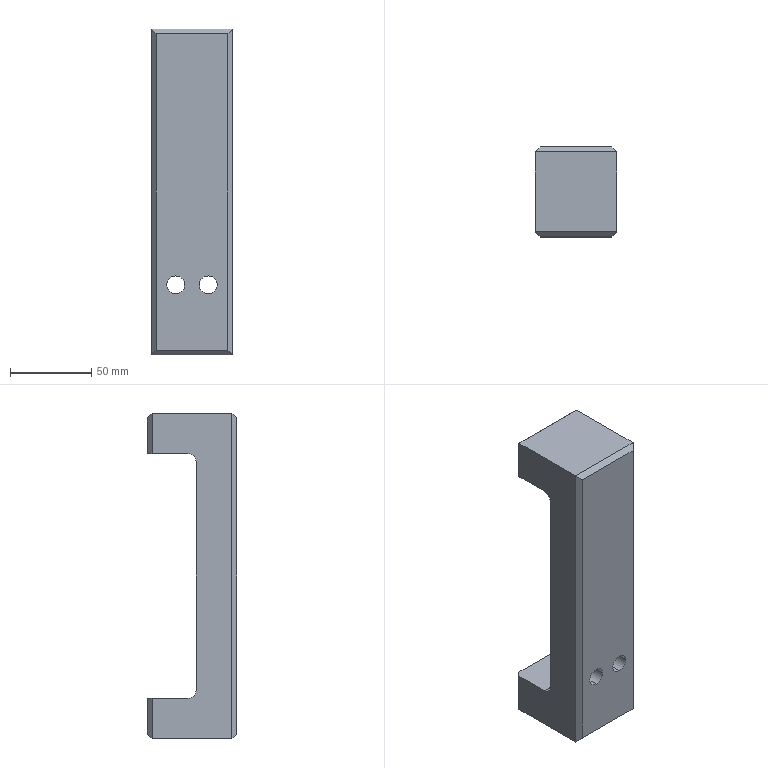Part | CATIA | 1 solid | 26 faces | box 50 x 55 x 200 mm | volume 317707 mm3 | plane 20 | cylinder 6 | commonest cylinder face diameters 11 x4 10 x2
STEP:
#1=CARTESIAN_POINT('',(-22.,-25.,172.));
#2=VERTEX_POINT('',#1);
#3=CARTESIAN_POINT('',(-25.,-22.,175.));
#4=VERTEX_POINT('',#3);
#5=CARTESIAN_POINT('',(-25.,-22.,175.));
#6=CARTESIAN_POINT('',(-22.,-25.,172.));
#7=B_SPLINE_CURVE_WITH_KNOTS('',1,(#5,#6),.UNSPECIFIED.,.F.,.U.,(2,2),(-2.598,2.598),.UNSPECIFIED.);
#8=EDGE_CURVE('',#2,#4,#7,.F.);
#9=ORIENTED_EDGE('',*,*,#8,.T.);
#10=CARTESIAN_POINT('',(-25.,-22.,-25.));
#11=VERTEX_POINT('',#10);
#12=CARTESIAN_POINT('',(-25.,-22.,75.));
#13=DIRECTION('',(0.,0.,1.));
#14=VECTOR('',#13,1.);
#15=LINE('',#12,#14);
#16=EDGE_CURVE('',#11,#4,#15,.T.);
#17=ORIENTED_EDGE('',*,*,#16,.F.);
#18=CARTESIAN_POINT('',(-22.,-25.,-22.));
#19=VERTEX_POINT('',#18);
#20=CARTESIAN_POINT('',(-25.,-22.,-25.));
#21=CARTESIAN_POINT('',(-22.,-25.,-22.));
#22=B_SPLINE_CURVE_WITH_KNOTS('',1,(#20,#21),.UNSPECIFIED.,.F.,.U.,(2,2),(-2.598,2.598),.UNSPECIFIED.);
#23=EDGE_CURVE('',#11,#19,#22,.T.);
#24=ORIENTED_EDGE('',*,*,#23,.T.);
#25=CARTESIAN_POINT('',(-22.,-25.,75.));
#26=DIRECTION('',(0.,0.,1.));
#27=VECTOR('',#26,1.);
#28=LINE('',#25,#27);
#29=EDGE_CURVE('',#19,#2,#28,.T.);
#30=ORIENTED_EDGE('',*,*,#29,.T.);
#31=EDGE_LOOP('',(#9,#17,#24,#30));
#32=FACE_OUTER_BOUND('',#31,.T.);
#33=CARTESIAN_POINT('',(-22.,-25.,-65.));
#34=DIRECTION('',(-0.7071,-0.7071,0.));
#35=DIRECTION('',(0.,0.,1.));
#36=AXIS2_PLACEMENT_3D('',#33,#34,#35);
#37=PLANE('',#36);
#38=ADVANCED_FACE('',(#32),#37,.T.);
#39=CARTESIAN_POINT('',(22.,-25.,172.));
#40=VERTEX_POINT('',#39);
#41=CARTESIAN_POINT('',(25.,-22.,175.));
#42=VERTEX_POINT('',#41);
#43=CARTESIAN_POINT('',(25.,-22.,175.));
#44=CARTESIAN_POINT('',(22.,-25.,172.));
#45=B_SPLINE_CURVE_WITH_KNOTS('',1,(#43,#44),.UNSPECIFIED.,.F.,.U.,(2,2),(-2.598,2.598),.UNSPECIFIED.);
#46=EDGE_CURVE('',#40,#42,#45,.F.);
#47=ORIENTED_EDGE('',*,*,#46,.T.);
#48=CARTESIAN_POINT('',(0.,-22.,175.));
#49=DIRECTION('',(1.,0.,0.));
#50=VECTOR('',#49,1.);
#51=LINE('',#48,#50);
#52=EDGE_CURVE('',#4,#42,#51,.T.);
#53=ORIENTED_EDGE('',*,*,#52,.F.);
#54=ORIENTED_EDGE('',*,*,#8,.F.);
#55=CARTESIAN_POINT('',(0.,-25.,172.));
#56=DIRECTION('',(1.,0.,0.));
#57=VECTOR('',#56,1.);
#58=LINE('',#55,#57);
#59=EDGE_CURVE('',#2,#40,#58,.T.);
#60=ORIENTED_EDGE('',*,*,#59,.T.);
#61=EDGE_LOOP('',(#47,#53,#54,#60));
#62=FACE_OUTER_BOUND('',#61,.T.);
#63=CARTESIAN_POINT('',(-35.,-25.,172.));
#64=DIRECTION('',(0.,-0.7071,0.7071));
#65=DIRECTION('',(1.,0.,0.));
#66=AXIS2_PLACEMENT_3D('',#63,#64,#65);
#67=PLANE('',#66);
#68=ADVANCED_FACE('',(#62),#67,.T.);
#69=CARTESIAN_POINT('',(25.,-22.,-25.));
#70=VERTEX_POINT('',#69);
#71=CARTESIAN_POINT('',(25.,-22.,75.));
#72=DIRECTION('',(0.,0.,1.));
#73=VECTOR('',#72,1.);
#74=LINE('',#71,#73);
#75=EDGE_CURVE('',#42,#70,#74,.F.);
#76=ORIENTED_EDGE('',*,*,#75,.F.);
#77=ORIENTED_EDGE('',*,*,#46,.F.);
#78=CARTESIAN_POINT('',(22.,-25.,-22.));
#79=VERTEX_POINT('',#78);
#80=CARTESIAN_POINT('',(22.,-25.,75.));
#81=DIRECTION('',(0.,0.,1.));
#82=VECTOR('',#81,1.);
#83=LINE('',#80,#82);
#84=EDGE_CURVE('',#40,#79,#83,.F.);
#85=ORIENTED_EDGE('',*,*,#84,.T.);
#86=CARTESIAN_POINT('',(25.,-22.,-25.));
#87=CARTESIAN_POINT('',(22.,-25.,-22.));
#88=B_SPLINE_CURVE_WITH_KNOTS('',1,(#86,#87),.UNSPECIFIED.,.F.,.U.,(2,2),(-2.598,2.598),.UNSPECIFIED.);
#89=EDGE_CURVE('',#79,#70,#88,.F.);
#90=ORIENTED_EDGE('',*,*,#89,.T.);
#91=EDGE_LOOP('',(#76,#77,#85,#90));
#92=FACE_OUTER_BOUND('',#91,.T.);
#93=CARTESIAN_POINT('',(22.,-25.,-65.));
#94=DIRECTION('',(-0.7071,0.7071,0.));
#95=DIRECTION('',(0.,0.,1.));
#96=AXIS2_PLACEMENT_3D('',#93,#94,#95);
#97=PLANE('',#96);
#98=ADVANCED_FACE('',(#92),#97,.F.);
#99=ORIENTED_EDGE('',*,*,#23,.F.);
#100=CARTESIAN_POINT('',(0.,-22.,-25.));
#101=DIRECTION('',(-1.,0.,0.));
#102=VECTOR('',#101,1.);
#103=LINE('',#100,#102);
#104=EDGE_CURVE('',#70,#11,#103,.T.);
#105=ORIENTED_EDGE('',*,*,#104,.F.);
#106=ORIENTED_EDGE('',*,*,#89,.F.);
#107=CARTESIAN_POINT('',(0.,-25.,-22.));
#108=DIRECTION('',(-1.,0.,0.));
#109=VECTOR('',#108,1.);
#110=LINE('',#107,#109);
#111=EDGE_CURVE('',#79,#19,#110,.T.);
#112=ORIENTED_EDGE('',*,*,#111,.T.);
#113=EDGE_LOOP('',(#99,#105,#106,#112));
#114=FACE_OUTER_BOUND('',#113,.T.);
#115=CARTESIAN_POINT('',(35.,-25.,-22.));
#116=DIRECTION('',(0.,-0.7071,-0.7071));
#117=DIRECTION('',(-1.,0.,0.));
#118=AXIS2_PLACEMENT_3D('',#115,#116,#117);
#119=PLANE('',#118);
#120=ADVANCED_FACE('',(#114),#119,.T.);
#121=CARTESIAN_POINT('',(-22.,30.,150.));
#122=VERTEX_POINT('',#121);
#123=CARTESIAN_POINT('',(22.,30.,150.));
#124=VERTEX_POINT('',#123);
#125=CARTESIAN_POINT('',(0.,30.,150.));
#126=DIRECTION('',(1.,0.,0.));
#127=VECTOR('',#126,1.);
#128=LINE('',#125,#127);
#129=EDGE_CURVE('',#122,#124,#128,.T.);
#130=ORIENTED_EDGE('',*,*,#129,.F.);
#131=CARTESIAN_POINT('',(-22.,30.,172.));
#132=VERTEX_POINT('',#131);
#133=CARTESIAN_POINT('',(-22.,30.,161.));
#134=DIRECTION('',(0.,0.,-1.));
#135=VECTOR('',#134,1.);
#136=LINE('',#133,#135);
#137=EDGE_CURVE('',#132,#122,#136,.T.);
#138=ORIENTED_EDGE('',*,*,#137,.F.);
#139=CARTESIAN_POINT('',(22.,30.,172.));
#140=VERTEX_POINT('',#139);
#141=CARTESIAN_POINT('',(0.,30.,172.));
#142=DIRECTION('',(-1.,0.,0.));
#143=VECTOR('',#142,1.);
#144=LINE('',#141,#143);
#145=EDGE_CURVE('',#140,#132,#144,.T.);
#146=ORIENTED_EDGE('',*,*,#145,.F.);
#147=CARTESIAN_POINT('',(22.,30.,161.));
#148=DIRECTION('',(0.,0.,-1.));
#149=VECTOR('',#148,1.);
#150=LINE('',#147,#149);
#151=EDGE_CURVE('',#124,#140,#150,.F.);
#152=ORIENTED_EDGE('',*,*,#151,.F.);
#153=EDGE_LOOP('',(#130,#138,#146,#152));
#154=FACE_OUTER_BOUND('',#153,.T.);
#155=CARTESIAN_POINT('',(0.,30.,-25.));
#156=DIRECTION('',(0.,1.,0.));
#157=DIRECTION('',(0.,0.,1.));
#158=AXIS2_PLACEMENT_3D('',#155,#156,#157);
#159=PLANE('',#158);
#160=ADVANCED_FACE('',(#154),#159,.T.);
#161=CARTESIAN_POINT('',(25.,27.,175.));
#162=VERTEX_POINT('',#161);
#163=CARTESIAN_POINT('',(-25.,27.,175.));
#164=VERTEX_POINT('',#163);
#165=CARTESIAN_POINT('',(0.,27.,175.));
#166=DIRECTION('',(-1.,0.,0.));
#167=VECTOR('',#166,1.);
#168=LINE('',#165,#167);
#169=EDGE_CURVE('',#162,#164,#168,.T.);
#170=ORIENTED_EDGE('',*,*,#169,.T.);
#171=CARTESIAN_POINT('',(-25.,2.5,175.));
#172=DIRECTION('',(0.,1.,0.));
#173=VECTOR('',#172,1.);
#174=LINE('',#171,#173);
#175=EDGE_CURVE('',#164,#4,#174,.F.);
#176=ORIENTED_EDGE('',*,*,#175,.T.);
#177=ORIENTED_EDGE('',*,*,#52,.T.);
#178=CARTESIAN_POINT('',(25.,2.5,175.));
#179=DIRECTION('',(0.,1.,0.));
#180=VECTOR('',#179,1.);
#181=LINE('',#178,#180);
#182=EDGE_CURVE('',#162,#42,#181,.F.);
#183=ORIENTED_EDGE('',*,*,#182,.F.);
#184=EDGE_LOOP('',(#170,#176,#177,#183));
#185=FACE_OUTER_BOUND('',#184,.T.);
#186=CARTESIAN_POINT('',(0.,-25.,175.));
#187=DIRECTION('',(0.,0.,-1.));
#188=DIRECTION('',(0.,1.,0.));
#189=AXIS2_PLACEMENT_3D('',#186,#187,#188);
#190=PLANE('',#189);
#191=ADVANCED_FACE('',(#185),#190,.F.);
#192=CARTESIAN_POINT('',(25.,27.,150.));
#193=VERTEX_POINT('',#192);
#194=CARTESIAN_POINT('',(25.,27.,75.));
#195=DIRECTION('',(0.,0.,-1.));
#196=VECTOR('',#195,1.);
#197=LINE('',#194,#196);
#198=EDGE_CURVE('',#193,#162,#197,.F.);
#199=ORIENTED_EDGE('',*,*,#198,.F.);
#200=CARTESIAN_POINT('',(23.5,28.5,150.));
#201=DIRECTION('',(0.7071,-0.7071,0.));
#202=VECTOR('',#201,1.);
#203=LINE('',#200,#202);
#204=EDGE_CURVE('',#193,#124,#203,.F.);
#205=ORIENTED_EDGE('',*,*,#204,.T.);
#206=ORIENTED_EDGE('',*,*,#151,.T.);
#207=CARTESIAN_POINT('',(25.,27.,175.));
#208=CARTESIAN_POINT('',(22.,30.,172.));
#209=B_SPLINE_CURVE_WITH_KNOTS('',1,(#207,#208),.UNSPECIFIED.,.F.,.U.,(2,2),(-2.598,2.598),.UNSPECIFIED.);
#210=EDGE_CURVE('',#140,#162,#209,.F.);
#211=ORIENTED_EDGE('',*,*,#210,.T.);
#212=EDGE_LOOP('',(#199,#205,#206,#211));
#213=FACE_OUTER_BOUND('',#212,.T.);
#214=CARTESIAN_POINT('',(22.,30.,215.));
#215=DIRECTION('',(-0.7071,-0.7071,0.));
#216=DIRECTION('',(0.,0.,-1.));
#217=AXIS2_PLACEMENT_3D('',#214,#215,#216);
#218=PLANE('',#217);
#219=ADVANCED_FACE('',(#213),#218,.F.);
#220=CARTESIAN_POINT('',(-25.,27.,175.));
#221=CARTESIAN_POINT('',(-22.,30.,172.));
#222=B_SPLINE_CURVE_WITH_KNOTS('',1,(#220,#221),.UNSPECIFIED.,.F.,.U.,(2,2),(-2.598,2.598),.UNSPECIFIED.);
#223=EDGE_CURVE('',#132,#164,#222,.F.);
#224=ORIENTED_EDGE('',*,*,#223,.T.);
#225=ORIENTED_EDGE('',*,*,#169,.F.);
#226=ORIENTED_EDGE('',*,*,#210,.F.);
#227=ORIENTED_EDGE('',*,*,#145,.T.);
#228=EDGE_LOOP('',(#224,#225,#226,#227));
#229=FACE_OUTER_BOUND('',#228,.T.);
#230=CARTESIAN_POINT('',(35.,30.,172.));
#231=DIRECTION('',(0.,0.7071,0.7071));
#232=DIRECTION('',(-1.,0.,0.));
#233=AXIS2_PLACEMENT_3D('',#230,#231,#232);
#234=PLANE('',#233);
#235=ADVANCED_FACE('',(#229),#234,.T.);
#236=CARTESIAN_POINT('',(-25.,27.,150.));
#237=VERTEX_POINT('',#236);
#238=CARTESIAN_POINT('',(-23.5,28.5,150.));
#239=DIRECTION('',(-0.7071,-0.7071,0.));
#240=VECTOR('',#239,1.);
#241=LINE('',#238,#240);
#242=EDGE_CURVE('',#122,#237,#241,.T.);
#243=ORIENTED_EDGE('',*,*,#242,.T.);
#244=CARTESIAN_POINT('',(-25.,27.,75.));
#245=DIRECTION('',(0.,0.,-1.));
#246=VECTOR('',#245,1.);
#247=LINE('',#244,#246);
#248=EDGE_CURVE('',#164,#237,#247,.T.);
#249=ORIENTED_EDGE('',*,*,#248,.F.);
#250=ORIENTED_EDGE('',*,*,#223,.F.);
#251=ORIENTED_EDGE('',*,*,#137,.T.);
#252=EDGE_LOOP('',(#243,#249,#250,#251));
#253=FACE_OUTER_BOUND('',#252,.T.);
#254=CARTESIAN_POINT('',(-22.,30.,215.));
#255=DIRECTION('',(-0.7071,0.7071,0.));
#256=DIRECTION('',(0.,0.,-1.));
#257=AXIS2_PLACEMENT_3D('',#254,#255,#256);
#258=PLANE('',#257);
#259=ADVANCED_FACE('',(#253),#258,.T.);
#260=CARTESIAN_POINT('',(-22.,30.,0.));
#261=VERTEX_POINT('',#260);
#262=CARTESIAN_POINT('',(22.,30.,0.));
#263=VERTEX_POINT('',#262);
#264=CARTESIAN_POINT('',(0.,30.,0.));
#265=DIRECTION('',(1.,0.,0.));
#266=VECTOR('',#265,1.);
#267=LINE('',#264,#266);
#268=EDGE_CURVE('',#261,#263,#267,.T.);
#269=ORIENTED_EDGE('',*,*,#268,.T.);
#270=CARTESIAN_POINT('',(22.,30.,-22.));
#271=VERTEX_POINT('',#270);
#272=CARTESIAN_POINT('',(22.,30.,-11.));
#273=DIRECTION('',(0.,0.,-1.));
#274=VECTOR('',#273,1.);
#275=LINE('',#272,#274);
#276=EDGE_CURVE('',#263,#271,#275,.T.);
#277=ORIENTED_EDGE('',*,*,#276,.T.);
#278=CARTESIAN_POINT('',(-22.,30.,-22.));
#279=VERTEX_POINT('',#278);
#280=CARTESIAN_POINT('',(0.,30.,-22.));
#281=DIRECTION('',(1.,0.,0.));
#282=VECTOR('',#281,1.);
#283=LINE('',#280,#282);
#284=EDGE_CURVE('',#271,#279,#283,.F.);
#285=ORIENTED_EDGE('',*,*,#284,.T.);
#286=CARTESIAN_POINT('',(-22.,30.,-11.));
#287=DIRECTION('',(0.,0.,-1.));
#288=VECTOR('',#287,1.);
#289=LINE('',#286,#288);
#290=EDGE_CURVE('',#279,#261,#289,.F.);
#291=ORIENTED_EDGE('',*,*,#290,.T.);
#292=EDGE_LOOP('',(#269,#277,#285,#291));
#293=FACE_OUTER_BOUND('',#292,.T.);
#294=ADVANCED_FACE('',(#293),#159,.T.);
#295=CARTESIAN_POINT('',(25.,27.,-25.));
#296=VERTEX_POINT('',#295);
#297=CARTESIAN_POINT('',(-25.,27.,-25.));
#298=VERTEX_POINT('',#297);
#299=CARTESIAN_POINT('',(0.,27.,-25.));
#300=DIRECTION('',(1.,0.,0.));
#301=VECTOR('',#300,1.);
#302=LINE('',#299,#301);
#303=EDGE_CURVE('',#296,#298,#302,.F.);
#304=ORIENTED_EDGE('',*,*,#303,.F.);
#305=CARTESIAN_POINT('',(25.,2.5,-25.));
#306=DIRECTION('',(0.,-1.,0.));
#307=VECTOR('',#306,1.);
#308=LINE('',#305,#307);
#309=EDGE_CURVE('',#70,#296,#308,.F.);
#310=ORIENTED_EDGE('',*,*,#309,.F.);
#311=ORIENTED_EDGE('',*,*,#104,.T.);
#312=CARTESIAN_POINT('',(-25.,2.5,-25.));
#313=DIRECTION('',(0.,-1.,0.));
#314=VECTOR('',#313,1.);
#315=LINE('',#312,#314);
#316=EDGE_CURVE('',#11,#298,#315,.F.);
#317=ORIENTED_EDGE('',*,*,#316,.T.);
#318=EDGE_LOOP('',(#304,#310,#311,#317));
#319=FACE_OUTER_BOUND('',#318,.T.);
#320=CARTESIAN_POINT('',(0.,30.,-25.));
#321=DIRECTION('',(0.,0.,1.));
#322=DIRECTION('',(0.,-1.,0.));
#323=AXIS2_PLACEMENT_3D('',#320,#321,#322);
#324=PLANE('',#323);
#325=ADVANCED_FACE('',(#319),#324,.F.);
#326=ORIENTED_EDGE('',*,*,#276,.F.);
#327=CARTESIAN_POINT('',(25.,27.,0.));
#328=VERTEX_POINT('',#327);
#329=CARTESIAN_POINT('',(23.5,28.5,0.));
#330=DIRECTION('',(0.7071,-0.7071,0.));
#331=VECTOR('',#330,1.);
#332=LINE('',#329,#331);
#333=EDGE_CURVE('',#263,#328,#332,.T.);
#334=ORIENTED_EDGE('',*,*,#333,.T.);
#335=CARTESIAN_POINT('',(25.,27.,75.));
#336=DIRECTION('',(0.,0.,-1.));
#337=VECTOR('',#336,1.);
#338=LINE('',#335,#337);
#339=EDGE_CURVE('',#328,#296,#338,.T.);
#340=ORIENTED_EDGE('',*,*,#339,.T.);
#341=CARTESIAN_POINT('',(25.,27.,-25.));
#342=CARTESIAN_POINT('',(22.,30.,-22.));
#343=B_SPLINE_CURVE_WITH_KNOTS('',1,(#341,#342),.UNSPECIFIED.,.F.,.U.,(2,2),(-2.598,2.598),.UNSPECIFIED.);
#344=EDGE_CURVE('',#296,#271,#343,.T.);
#345=ORIENTED_EDGE('',*,*,#344,.T.);
#346=EDGE_LOOP('',(#326,#334,#340,#345));
#347=FACE_OUTER_BOUND('',#346,.T.);
#348=CARTESIAN_POINT('',(22.,30.,215.));
#349=DIRECTION('',(-0.7071,-0.7071,0.));
#350=DIRECTION('',(0.,0.,-1.));
#351=AXIS2_PLACEMENT_3D('',#348,#349,#350);
#352=PLANE('',#351);
#353=ADVANCED_FACE('',(#347),#352,.F.);
#354=CARTESIAN_POINT('',(-25.,27.,-25.));
#355=CARTESIAN_POINT('',(-22.,30.,-22.));
#356=B_SPLINE_CURVE_WITH_KNOTS('',1,(#354,#355),.UNSPECIFIED.,.F.,.U.,(2,2),(-2.598,2.598),.UNSPECIFIED.);
#357=EDGE_CURVE('',#298,#279,#356,.T.);
#358=ORIENTED_EDGE('',*,*,#357,.T.);
#359=ORIENTED_EDGE('',*,*,#284,.F.);
#360=ORIENTED_EDGE('',*,*,#344,.F.);
#361=ORIENTED_EDGE('',*,*,#303,.T.);
#362=EDGE_LOOP('',(#358,#359,#360,#361));
#363=FACE_OUTER_BOUND('',#362,.T.);
#364=CARTESIAN_POINT('',(-35.,30.,-22.));
#365=DIRECTION('',(0.,0.7071,-0.7071));
#366=DIRECTION('',(1.,0.,0.));
#367=AXIS2_PLACEMENT_3D('',#364,#365,#366);
#368=PLANE('',#367);
#369=ADVANCED_FACE('',(#363),#368,.T.);
#370=CARTESIAN_POINT('',(-25.,27.,0.));
#371=VERTEX_POINT('',#370);
#372=CARTESIAN_POINT('',(-23.5,28.5,0.));
#373=DIRECTION('',(-0.7071,-0.7071,0.));
#374=VECTOR('',#373,1.);
#375=LINE('',#372,#374);
#376=EDGE_CURVE('',#371,#261,#375,.F.);
#377=ORIENTED_EDGE('',*,*,#376,.T.);
#378=ORIENTED_EDGE('',*,*,#290,.F.);
#379=ORIENTED_EDGE('',*,*,#357,.F.);
#380=CARTESIAN_POINT('',(-25.,27.,75.));
#381=DIRECTION('',(0.,0.,-1.));
#382=VECTOR('',#381,1.);
#383=LINE('',#380,#382);
#384=EDGE_CURVE('',#298,#371,#383,.F.);
#385=ORIENTED_EDGE('',*,*,#384,.T.);
#386=EDGE_LOOP('',(#377,#378,#379,#385));
#387=FACE_OUTER_BOUND('',#386,.T.);
#388=CARTESIAN_POINT('',(-22.,30.,215.));
#389=DIRECTION('',(-0.7071,0.7071,0.));
#390=DIRECTION('',(0.,0.,-1.));
#391=AXIS2_PLACEMENT_3D('',#388,#389,#390);
#392=PLANE('',#391);
#393=ADVANCED_FACE('',(#387),#392,.T.);
#394=CARTESIAN_POINT('',(25.,5.,0.));
#395=VERTEX_POINT('',#394);
#396=CARTESIAN_POINT('',(25.,16.,0.));
#397=DIRECTION('',(0.,-1.,0.));
#398=VECTOR('',#397,1.);
#399=LINE('',#396,#398);
#400=EDGE_CURVE('',#328,#395,#399,.T.);
#401=ORIENTED_EDGE('',*,*,#400,.F.);
#402=ORIENTED_EDGE('',*,*,#333,.F.);
#403=ORIENTED_EDGE('',*,*,#268,.F.);
#404=ORIENTED_EDGE('',*,*,#376,.F.);
#405=CARTESIAN_POINT('',(-25.,5.,0.));
#406=VERTEX_POINT('',#405);
#407=CARTESIAN_POINT('',(-25.,16.,0.));
#408=DIRECTION('',(0.,-1.,0.));
#409=VECTOR('',#408,1.);
#410=LINE('',#407,#409);
#411=EDGE_CURVE('',#371,#406,#410,.T.);
#412=ORIENTED_EDGE('',*,*,#411,.T.);
#413=CARTESIAN_POINT('',(0.,5.,0.));
#414=DIRECTION('',(1.,0.,0.));
#415=VECTOR('',#414,1.);
#416=LINE('',#413,#415);
#417=EDGE_CURVE('',#395,#406,#416,.F.);
#418=ORIENTED_EDGE('',*,*,#417,.F.);
#419=EDGE_LOOP('',(#401,#402,#403,#404,#412,#418));
#420=FACE_OUTER_BOUND('',#419,.T.);
#421=CARTESIAN_POINT('',(0.,30.,0.));
#422=DIRECTION('',(0.,0.,1.));
#423=DIRECTION('',(0.,-1.,0.));
#424=AXIS2_PLACEMENT_3D('',#421,#422,#423);
#425=PLANE('',#424);
#426=ADVANCED_FACE('',(#420),#425,.T.);
#427=CARTESIAN_POINT('',(25.,0.,5.));
#428=VERTEX_POINT('',#427);
#429=CARTESIAN_POINT('',(-25.,0.,5.));
#430=VERTEX_POINT('',#429);
#431=CARTESIAN_POINT('',(0.,0.,5.));
#432=DIRECTION('',(1.,0.,0.));
#433=VECTOR('',#432,1.);
#434=LINE('',#431,#433);
#435=EDGE_CURVE('',#428,#430,#434,.F.);
#436=ORIENTED_EDGE('',*,*,#435,.F.);
#437=CARTESIAN_POINT('',(25.,5.,5.));
#438=DIRECTION('',(1.,0.,0.));
#439=AXIS2_PLACEMENT_3D('',#437,#438,$);
#440=CIRCLE('',#439,5.);
#441=EDGE_CURVE('',#395,#428,#440,.F.);
#442=ORIENTED_EDGE('',*,*,#441,.F.);
#443=ORIENTED_EDGE('',*,*,#417,.T.);
#444=CARTESIAN_POINT('',(-25.,5.,5.));
#445=DIRECTION('',(1.,0.,0.));
#446=AXIS2_PLACEMENT_3D('',#444,#445,$);
#447=CIRCLE('',#446,5.);
#448=EDGE_CURVE('',#430,#406,#447,.T.);
#449=ORIENTED_EDGE('',*,*,#448,.F.);
#450=EDGE_LOOP('',(#436,#442,#443,#449));
#451=FACE_OUTER_BOUND('',#450,.T.);
#452=CARTESIAN_POINT('',(0.,5.,5.));
#453=DIRECTION('',(1.,0.,0.));
#454=DIRECTION('',(0.,-1.,0.));
#455=AXIS2_PLACEMENT_3D('',#452,#453,#454);
#456=CYLINDRICAL_SURFACE('',#455,5.);
#457=ADVANCED_FACE('',(#451),#456,.F.);
#458=CARTESIAN_POINT('',(25.,0.,145.));
#459=VERTEX_POINT('',#458);
#460=CARTESIAN_POINT('',(25.,5.,150.));
#461=VERTEX_POINT('',#460);
#462=CARTESIAN_POINT('',(25.,5.,145.));
#463=DIRECTION('',(1.,0.,0.));
#464=AXIS2_PLACEMENT_3D('',#462,#463,$);
#465=CIRCLE('',#464,5.);
#466=EDGE_CURVE('',#459,#461,#465,.F.);
#467=ORIENTED_EDGE('',*,*,#466,.T.);
#468=CARTESIAN_POINT('',(25.,16.,150.));
#469=DIRECTION('',(0.,1.,0.));
#470=VECTOR('',#469,1.);
#471=LINE('',#468,#470);
#472=EDGE_CURVE('',#461,#193,#471,.T.);
#473=ORIENTED_EDGE('',*,*,#472,.T.);
#474=ORIENTED_EDGE('',*,*,#198,.T.);
#475=ORIENTED_EDGE('',*,*,#182,.T.);
#476=ORIENTED_EDGE('',*,*,#75,.T.);
#477=ORIENTED_EDGE('',*,*,#309,.T.);
#478=ORIENTED_EDGE('',*,*,#339,.F.);
#479=ORIENTED_EDGE('',*,*,#400,.T.);
#480=ORIENTED_EDGE('',*,*,#441,.T.);
#481=CARTESIAN_POINT('',(25.,0.,75.));
#482=DIRECTION('',(0.,0.,-1.));
#483=VECTOR('',#482,1.);
#484=LINE('',#481,#483);
#485=EDGE_CURVE('',#428,#459,#484,.F.);
#486=ORIENTED_EDGE('',*,*,#485,.T.);
#487=EDGE_LOOP('',(#467,#473,#474,#475,#476,#477,#478,#479,#480,#486));
#488=FACE_OUTER_BOUND('',#487,.T.);
#489=CARTESIAN_POINT('',(25.,0.,0.));
#490=DIRECTION('',(1.,0.,0.));
#491=DIRECTION('',(0.,1.,0.));
#492=AXIS2_PLACEMENT_3D('',#489,#490,#491);
#493=PLANE('',#492);
#494=ADVANCED_FACE('',(#488),#493,.T.);
#495=CARTESIAN_POINT('',(-25.,0.,145.));
#496=VERTEX_POINT('',#495);
#497=CARTESIAN_POINT('',(-25.,0.,75.));
#498=DIRECTION('',(0.,0.,-1.));
#499=VECTOR('',#498,1.);
#500=LINE('',#497,#499);
#501=EDGE_CURVE('',#430,#496,#500,.F.);
#502=ORIENTED_EDGE('',*,*,#501,.F.);
#503=ORIENTED_EDGE('',*,*,#448,.T.);
#504=ORIENTED_EDGE('',*,*,#411,.F.);
#505=ORIENTED_EDGE('',*,*,#384,.F.);
#506=ORIENTED_EDGE('',*,*,#316,.F.);
#507=ORIENTED_EDGE('',*,*,#16,.T.);
#508=ORIENTED_EDGE('',*,*,#175,.F.);
#509=ORIENTED_EDGE('',*,*,#248,.T.);
#510=CARTESIAN_POINT('',(-25.,5.,150.));
#511=VERTEX_POINT('',#510);
#512=CARTESIAN_POINT('',(-25.,16.,150.));
#513=DIRECTION('',(0.,1.,0.));
#514=VECTOR('',#513,1.);
#515=LINE('',#512,#514);
#516=EDGE_CURVE('',#511,#237,#515,.T.);
#517=ORIENTED_EDGE('',*,*,#516,.F.);
#518=CARTESIAN_POINT('',(-25.,5.,145.));
#519=DIRECTION('',(1.,0.,0.));
#520=AXIS2_PLACEMENT_3D('',#518,#519,$);
#521=CIRCLE('',#520,5.);
#522=EDGE_CURVE('',#511,#496,#521,.T.);
#523=ORIENTED_EDGE('',*,*,#522,.T.);
#524=EDGE_LOOP('',(#502,#503,#504,#505,#506,#507,#508,#509,#517,#523));
#525=FACE_OUTER_BOUND('',#524,.T.);
#526=CARTESIAN_POINT('',(-25.,0.,0.));
#527=DIRECTION('',(1.,0.,0.));
#528=DIRECTION('',(0.,1.,0.));
#529=AXIS2_PLACEMENT_3D('',#526,#527,#528);
#530=PLANE('',#529);
#531=ADVANCED_FACE('',(#525),#530,.F.);
#532=ORIENTED_EDGE('',*,*,#516,.T.);
#533=ORIENTED_EDGE('',*,*,#242,.F.);
#534=ORIENTED_EDGE('',*,*,#129,.T.);
#535=ORIENTED_EDGE('',*,*,#204,.F.);
#536=ORIENTED_EDGE('',*,*,#472,.F.);
#537=CARTESIAN_POINT('',(0.,5.,150.));
#538=DIRECTION('',(1.,0.,0.));
#539=VECTOR('',#538,1.);
#540=LINE('',#537,#539);
#541=EDGE_CURVE('',#461,#511,#540,.F.);
#542=ORIENTED_EDGE('',*,*,#541,.T.);
#543=EDGE_LOOP('',(#532,#533,#534,#535,#536,#542));
#544=FACE_OUTER_BOUND('',#543,.T.);
#545=CARTESIAN_POINT('',(0.,0.,150.));
#546=DIRECTION('',(0.,0.,-1.));
#547=DIRECTION('',(0.,1.,0.));
#548=AXIS2_PLACEMENT_3D('',#545,#546,#547);
#549=PLANE('',#548);
#550=ADVANCED_FACE('',(#544),#549,.T.);
#551=ORIENTED_EDGE('',*,*,#541,.F.);
#552=ORIENTED_EDGE('',*,*,#466,.F.);
#553=CARTESIAN_POINT('',(0.,0.,145.));
#554=DIRECTION('',(1.,0.,0.));
#555=VECTOR('',#554,1.);
#556=LINE('',#553,#555);
#557=EDGE_CURVE('',#459,#496,#556,.F.);
#558=ORIENTED_EDGE('',*,*,#557,.T.);
#559=ORIENTED_EDGE('',*,*,#522,.F.);
#560=EDGE_LOOP('',(#551,#552,#558,#559));
#561=FACE_OUTER_BOUND('',#560,.T.);
#562=CARTESIAN_POINT('',(0.,5.,145.));
#563=DIRECTION('',(1.,0.,0.));
#564=DIRECTION('',(0.,0.,1.));
#565=AXIS2_PLACEMENT_3D('',#562,#563,#564);
#566=CYLINDRICAL_SURFACE('',#565,5.);
#567=ADVANCED_FACE('',(#561),#566,.F.);
#568=ORIENTED_EDGE('',*,*,#557,.F.);
#569=ORIENTED_EDGE('',*,*,#485,.F.);
#570=ORIENTED_EDGE('',*,*,#435,.T.);
#571=ORIENTED_EDGE('',*,*,#501,.T.);
#572=EDGE_LOOP('',(#568,#569,#570,#571));
#573=FACE_OUTER_BOUND('',#572,.T.);
#574=CARTESIAN_POINT('',(-10.,0.,12.5));
#575=VERTEX_POINT('',#574);
#576=CARTESIAN_POINT('',(-10.,0.,23.5));
#577=VERTEX_POINT('',#576);
#578=CARTESIAN_POINT('',(-10.,0.,18.));
#579=DIRECTION('',(0.,-1.,0.));
#580=AXIS2_PLACEMENT_3D('',#578,#579,$);
#581=CIRCLE('',#580,5.5);
#582=EDGE_CURVE('',#575,#577,#581,.F.);
#583=ORIENTED_EDGE('',*,*,#582,.F.);
#584=CARTESIAN_POINT('',(-10.,0.,18.));
#585=DIRECTION('',(0.,-1.,0.));
#586=AXIS2_PLACEMENT_3D('',#584,#585,$);
#587=CIRCLE('',#586,5.5);
#588=EDGE_CURVE('',#577,#575,#587,.F.);
#589=ORIENTED_EDGE('',*,*,#588,.F.);
#590=EDGE_LOOP('',(#583,#589));
#591=FACE_BOUND('',#590,.T.);
#592=CARTESIAN_POINT('',(10.,0.,12.5));
#593=VERTEX_POINT('',#592);
#594=CARTESIAN_POINT('',(10.,0.,23.5));
#595=VERTEX_POINT('',#594);
#596=CARTESIAN_POINT('',(10.,0.,18.));
#597=DIRECTION('',(0.,-1.,0.));
#598=AXIS2_PLACEMENT_3D('',#596,#597,$);
#599=CIRCLE('',#598,5.5);
#600=EDGE_CURVE('',#593,#595,#599,.F.);
#601=ORIENTED_EDGE('',*,*,#600,.F.);
#602=CARTESIAN_POINT('',(10.,0.,18.));
#603=DIRECTION('',(0.,-1.,0.));
#604=AXIS2_PLACEMENT_3D('',#602,#603,$);
#605=CIRCLE('',#604,5.5);
#606=EDGE_CURVE('',#595,#593,#605,.F.);
#607=ORIENTED_EDGE('',*,*,#606,.F.);
#608=EDGE_LOOP('',(#601,#607));
#609=FACE_BOUND('',#608,.T.);
#610=CARTESIAN_POINT('',(0.,0.,150.));
#611=DIRECTION('',(0.,-1.,0.));
#612=DIRECTION('',(0.,0.,-1.));
#613=AXIS2_PLACEMENT_3D('',#610,#611,#612);
#614=PLANE('',#613);
#615=ADVANCED_FACE('',(#573,#591,#609),#614,.F.);
#616=ORIENTED_EDGE('',*,*,#29,.F.);
#617=ORIENTED_EDGE('',*,*,#111,.F.);
#618=ORIENTED_EDGE('',*,*,#84,.F.);
#619=ORIENTED_EDGE('',*,*,#59,.F.);
#620=EDGE_LOOP('',(#616,#617,#618,#619));
#621=FACE_OUTER_BOUND('',#620,.T.);
#622=CARTESIAN_POINT('',(-10.,-25.,23.5));
#623=VERTEX_POINT('',#622);
#624=CARTESIAN_POINT('',(-10.,-25.,12.5));
#625=VERTEX_POINT('',#624);
#626=CARTESIAN_POINT('',(-10.,-25.,18.));
#627=DIRECTION('',(0.,-1.,0.));
#628=AXIS2_PLACEMENT_3D('',#626,#627,$);
#629=CIRCLE('',#628,5.5);
#630=EDGE_CURVE('',#623,#625,#629,.T.);
#631=ORIENTED_EDGE('',*,*,#630,.F.);
#632=CARTESIAN_POINT('',(-10.,-25.,18.));
#633=DIRECTION('',(0.,-1.,0.));
#634=AXIS2_PLACEMENT_3D('',#632,#633,$);
#635=CIRCLE('',#634,5.5);
#636=EDGE_CURVE('',#625,#623,#635,.T.);
#637=ORIENTED_EDGE('',*,*,#636,.F.);
#638=EDGE_LOOP('',(#631,#637));
#639=FACE_BOUND('',#638,.T.);
#640=CARTESIAN_POINT('',(10.,-25.,23.5));
#641=VERTEX_POINT('',#640);
#642=CARTESIAN_POINT('',(10.,-25.,12.5));
#643=VERTEX_POINT('',#642);
#644=CARTESIAN_POINT('',(10.,-25.,18.));
#645=DIRECTION('',(0.,-1.,0.));
#646=AXIS2_PLACEMENT_3D('',#644,#645,$);
#647=CIRCLE('',#646,5.5);
#648=EDGE_CURVE('',#641,#643,#647,.T.);
#649=ORIENTED_EDGE('',*,*,#648,.F.);
#650=CARTESIAN_POINT('',(10.,-25.,18.));
#651=DIRECTION('',(0.,-1.,0.));
#652=AXIS2_PLACEMENT_3D('',#650,#651,$);
#653=CIRCLE('',#652,5.5);
#654=EDGE_CURVE('',#643,#641,#653,.T.);
#655=ORIENTED_EDGE('',*,*,#654,.F.);
#656=EDGE_LOOP('',(#649,#655));
#657=FACE_BOUND('',#656,.T.);
#658=CARTESIAN_POINT('',(0.,-25.,175.));
#659=DIRECTION('',(0.,-1.,0.));
#660=DIRECTION('',(0.,0.,-1.));
#661=AXIS2_PLACEMENT_3D('',#658,#659,#660);
#662=PLANE('',#661);
#663=ADVANCED_FACE('',(#621,#639,#657),#662,.T.);
#664=ORIENTED_EDGE('',*,*,#654,.T.);
#665=CARTESIAN_POINT('',(10.,-13.11,23.5));
#666=DIRECTION('',(0.,1.,0.));
#667=VECTOR('',#666,1.);
#668=LINE('',#665,#667);
#669=EDGE_CURVE('',#595,#641,#668,.F.);
#670=ORIENTED_EDGE('',*,*,#669,.F.);
#671=ORIENTED_EDGE('',*,*,#606,.T.);
#672=CARTESIAN_POINT('',(10.,-13.11,12.5));
#673=DIRECTION('',(0.,1.,0.));
#674=VECTOR('',#673,1.);
#675=LINE('',#672,#674);
#676=EDGE_CURVE('',#593,#643,#675,.F.);
#677=ORIENTED_EDGE('',*,*,#676,.T.);
#678=EDGE_LOOP('',(#664,#670,#671,#677));
#679=FACE_OUTER_BOUND('',#678,.T.);
#680=CARTESIAN_POINT('',(10.,-13.11,18.));
#681=DIRECTION('',(0.,1.,0.));
#682=DIRECTION('',(0.,0.,1.));
#683=AXIS2_PLACEMENT_3D('',#680,#681,#682);
#684=CYLINDRICAL_SURFACE('',#683,5.5);
#685=ADVANCED_FACE('',(#679),#684,.F.);
#686=ORIENTED_EDGE('',*,*,#648,.T.);
#687=ORIENTED_EDGE('',*,*,#676,.F.);
#688=ORIENTED_EDGE('',*,*,#600,.T.);
#689=ORIENTED_EDGE('',*,*,#669,.T.);
#690=EDGE_LOOP('',(#686,#687,#688,#689));
#691=FACE_OUTER_BOUND('',#690,.T.);
#692=ADVANCED_FACE('',(#691),#684,.F.);
#693=ORIENTED_EDGE('',*,*,#636,.T.);
#694=CARTESIAN_POINT('',(-10.,-13.11,23.5));
#695=DIRECTION('',(0.,1.,0.));
#696=VECTOR('',#695,1.);
#697=LINE('',#694,#696);
#698=EDGE_CURVE('',#577,#623,#697,.F.);
#699=ORIENTED_EDGE('',*,*,#698,.F.);
#700=ORIENTED_EDGE('',*,*,#588,.T.);
#701=CARTESIAN_POINT('',(-10.,-13.11,12.5));
#702=DIRECTION('',(0.,1.,0.));
#703=VECTOR('',#702,1.);
#704=LINE('',#701,#703);
#705=EDGE_CURVE('',#575,#625,#704,.F.);
#706=ORIENTED_EDGE('',*,*,#705,.T.);
#707=EDGE_LOOP('',(#693,#699,#700,#706));
#708=FACE_OUTER_BOUND('',#707,.T.);
#709=CARTESIAN_POINT('',(-10.,-13.11,18.));
#710=DIRECTION('',(0.,1.,0.));
#711=DIRECTION('',(0.,0.,1.));
#712=AXIS2_PLACEMENT_3D('',#709,#710,#711);
#713=CYLINDRICAL_SURFACE('',#712,5.5);
#714=ADVANCED_FACE('',(#708),#713,.F.);
#715=ORIENTED_EDGE('',*,*,#630,.T.);
#716=ORIENTED_EDGE('',*,*,#705,.F.);
#717=ORIENTED_EDGE('',*,*,#582,.T.);
#718=ORIENTED_EDGE('',*,*,#698,.T.);
#719=EDGE_LOOP('',(#715,#716,#717,#718));
#720=FACE_OUTER_BOUND('',#719,.T.);
#721=ADVANCED_FACE('',(#720),#713,.F.);
#722=CLOSED_SHELL('',(#38,#68,#98,#120,#160,#191,#219,#235,#259,#294,#325,#353,#369,#393,#426,#457,#494,#531,#550,#567,#615,#663,#685,#692,#714,#721));
#723=MANIFOLD_SOLID_BREP('',#722);
#724=(LENGTH_UNIT()NAMED_UNIT(*)SI_UNIT(.MILLI.,.METRE.));
#725=UNCERTAINTY_MEASURE_WITH_UNIT(LENGTH_MEASURE(0.005),#724,'','');
#726=(NAMED_UNIT(*)PLANE_ANGLE_UNIT()SI_UNIT($,.RADIAN.));
#727=(NAMED_UNIT(*)SI_UNIT($,.STERADIAN.)SOLID_ANGLE_UNIT());
#728=(GEOMETRIC_REPRESENTATION_CONTEXT(3)GLOBAL_UNCERTAINTY_ASSIGNED_CONTEXT((#725))GLOBAL_UNIT_ASSIGNED_CONTEXT((#724,#726,#727))REPRESENTATION_CONTEXT('',''));
#729=ADVANCED_BREP_SHAPE_REPRESENTATION('',(#723),#728);